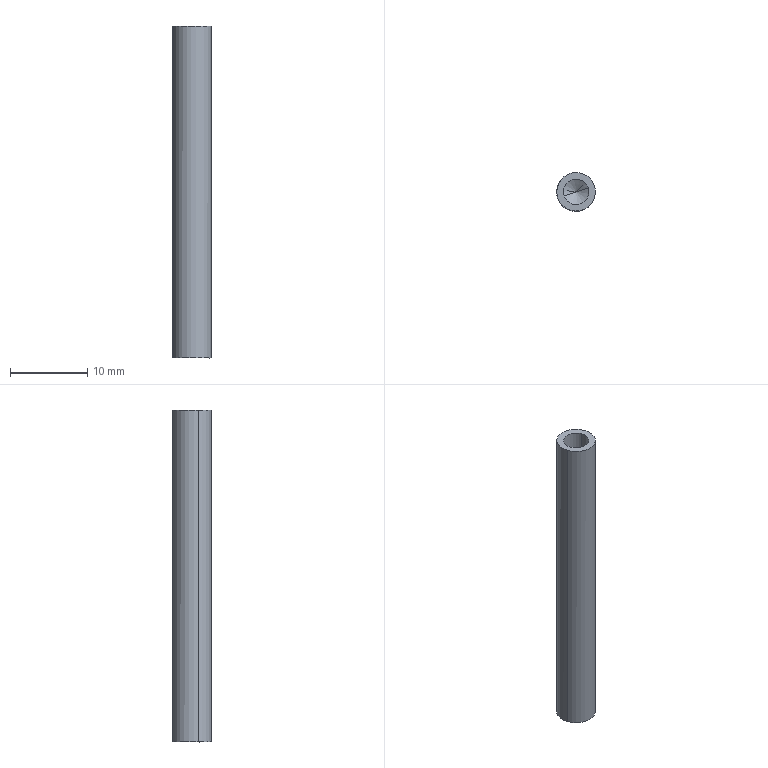Part | SolidWorks | features BaseBody 1 | 1 solid | 12 faces | box 5.036 x 5.019 x 43.005 mm | volume 701.802 mm3 | cylinder 6 | cone 4 | plane 2 | commonest cylinder face diameters 3.3 x4 5 x2
STEP:
#1=CARTESIAN_POINT('',(-258.909,167.447,-138.014));
#2=VERTEX_POINT('',#1);
#3=CARTESIAN_POINT('',(-260.471,166.914,-139.005));
#4=VERTEX_POINT('',#3);
#5=CARTESIAN_POINT('',(-258.909,167.447,-138.014));
#6=DIRECTION('',(-0.8116,-0.2768,-0.5145));
#7=VECTOR('',#6,1000.);
#8=LINE('',#5,#7);
#9=EDGE_CURVE('',#2,#4,#8,.T.);
#10=ORIENTED_EDGE('',*,*,#9,.F.);
#11=CARTESIAN_POINT('',(-262.031,166.381,-138.012));
#12=VERTEX_POINT('',#11);
#13=CARTESIAN_POINT('',(-260.47,166.914,-138.013));
#14=DIRECTION('',(-0.0008339,0.0004454,-1.));
#15=DIRECTION('',(-0.9463,-0.3232,0.0006452));
#16=AXIS2_PLACEMENT_3D('',#13,#14,#15);
#17=CIRCLE('',#16,1.65);
#18=EDGE_CURVE('',#12,#2,#17,.T.);
#19=ORIENTED_EDGE('',*,*,#18,.F.);
#20=CARTESIAN_POINT('',(-262.031,166.381,-138.012));
#21=DIRECTION('',(0.8107,0.2773,-0.5156));
#22=VECTOR('',#21,1000.);
#23=LINE('',#20,#22);
#24=EDGE_CURVE('',#12,#4,#23,.T.);
#25=ORIENTED_EDGE('',*,*,#24,.T.);
#26=EDGE_LOOP('',(#10,#19,#25));
#27=FACE_OUTER_BOUND('',#26,.T.);
#28=CARTESIAN_POINT('',(-260.47,166.914,-138.478));
#29=DIRECTION('',(0.0008339,-0.0004454,1.));
#30=DIRECTION('',(0.9463,0.3232,-0.0006452));
#31=AXIS2_PLACEMENT_3D('',#28,#29,#30);
#32=CONICAL_SURFACE('',#31,0.8764,1.03);
#33=ADVANCED_FACE('',(#27),#32,.F.);
#34=ORIENTED_EDGE('',*,*,#24,.F.);
#35=CARTESIAN_POINT('',(-260.47,166.914,-138.013));
#36=DIRECTION('',(-0.0008339,0.0004454,-1.));
#37=DIRECTION('',(0.9463,0.3232,-0.0006452));
#38=AXIS2_PLACEMENT_3D('',#35,#36,#37);
#39=CIRCLE('',#38,1.65);
#40=EDGE_CURVE('',#2,#12,#39,.T.);
#41=ORIENTED_EDGE('',*,*,#40,.F.);
#42=ORIENTED_EDGE('',*,*,#9,.T.);
#43=EDGE_LOOP('',(#34,#41,#42));
#44=FACE_OUTER_BOUND('',#43,.T.);
#45=CARTESIAN_POINT('',(-260.47,166.914,-138.478));
#46=DIRECTION('',(0.0008339,-0.0004454,1.));
#47=DIRECTION('',(0.9463,0.3232,-0.0006452));
#48=AXIS2_PLACEMENT_3D('',#45,#46,#47);
#49=CONICAL_SURFACE('',#48,0.8764,1.03);
#50=ADVANCED_FACE('',(#44),#49,.F.);
#51=CARTESIAN_POINT('',(-262.025,166.377,-130.012));
#52=VERTEX_POINT('',#51);
#53=CARTESIAN_POINT('',(-262.025,166.377,-130.012));
#54=DIRECTION('',(-0.0008339,0.0004454,-1.));
#55=VECTOR('',#54,1000.);
#56=LINE('',#53,#55);
#57=EDGE_CURVE('',#52,#12,#56,.T.);
#58=ORIENTED_EDGE('',*,*,#57,.F.);
#59=CARTESIAN_POINT('',(-258.902,167.444,-130.014));
#60=VERTEX_POINT('',#59);
#61=CARTESIAN_POINT('',(-260.463,166.91,-130.013));
#62=DIRECTION('',(0.0008339,-0.0004454,1.));
#63=DIRECTION('',(-0.9463,-0.3232,0.0006452));
#64=AXIS2_PLACEMENT_3D('',#61,#62,#63);
#65=CIRCLE('',#64,1.65);
#66=EDGE_CURVE('',#52,#60,#65,.T.);
#67=ORIENTED_EDGE('',*,*,#66,.T.);
#68=CARTESIAN_POINT('',(-258.902,167.444,-130.014));
#69=DIRECTION('',(-0.0008339,0.0004454,-1.));
#70=VECTOR('',#69,1000.);
#71=LINE('',#68,#70);
#72=EDGE_CURVE('',#60,#2,#71,.T.);
#73=ORIENTED_EDGE('',*,*,#72,.T.);
#74=ORIENTED_EDGE('',*,*,#40,.T.);
#75=EDGE_LOOP('',(#58,#67,#73,#74));
#76=FACE_OUTER_BOUND('',#75,.T.);
#77=CARTESIAN_POINT('',(-260.463,166.91,-130.013));
#78=DIRECTION('',(0.0008339,-0.0004454,1.));
#79=DIRECTION('',(0.9463,0.3232,-0.0006452));
#80=AXIS2_PLACEMENT_3D('',#77,#78,#79);
#81=CYLINDRICAL_SURFACE('',#80,1.65);
#82=ADVANCED_FACE('',(#76),#81,.F.);
#83=ORIENTED_EDGE('',*,*,#18,.T.);
#84=ORIENTED_EDGE('',*,*,#72,.F.);
#85=CARTESIAN_POINT('',(-260.463,166.91,-130.013));
#86=DIRECTION('',(0.0008339,-0.0004454,1.));
#87=DIRECTION('',(0.9463,0.3232,-0.0006452));
#88=AXIS2_PLACEMENT_3D('',#85,#86,#87);
#89=CIRCLE('',#88,1.65);
#90=EDGE_CURVE('',#60,#52,#89,.T.);
#91=ORIENTED_EDGE('',*,*,#90,.T.);
#92=ORIENTED_EDGE('',*,*,#57,.T.);
#93=EDGE_LOOP('',(#83,#84,#91,#92));
#94=FACE_OUTER_BOUND('',#93,.T.);
#95=CARTESIAN_POINT('',(-260.463,166.91,-130.013));
#96=DIRECTION('',(0.0008339,-0.0004454,1.));
#97=DIRECTION('',(0.9463,0.3232,-0.0006452));
#98=AXIS2_PLACEMENT_3D('',#95,#96,#97);
#99=CYLINDRICAL_SURFACE('',#98,1.65);
#100=ADVANCED_FACE('',(#94),#99,.F.);
#101=ORIENTED_EDGE('',*,*,#66,.F.);
#102=ORIENTED_EDGE('',*,*,#90,.F.);
#103=EDGE_LOOP('',(#101,#102));
#104=FACE_BOUND('',#103,.T.);
#105=CARTESIAN_POINT('',(-262.829,166.102,-130.011));
#106=VERTEX_POINT('',#105);
#107=CARTESIAN_POINT('',(-258.098,167.718,-130.015));
#108=VERTEX_POINT('',#107);
#109=CARTESIAN_POINT('',(-260.463,166.91,-130.013));
#110=DIRECTION('',(-0.0008339,0.0004454,-1.));
#111=DIRECTION('',(-0.9463,-0.3232,0.0006452));
#112=AXIS2_PLACEMENT_3D('',#109,#110,#111);
#113=CIRCLE('',#112,2.5);
#114=EDGE_CURVE('',#106,#108,#113,.T.);
#115=ORIENTED_EDGE('',*,*,#114,.F.);
#116=CARTESIAN_POINT('',(-260.463,166.91,-130.013));
#117=DIRECTION('',(-0.0008339,0.0004454,-1.));
#118=DIRECTION('',(0.9463,0.3232,-0.0006452));
#119=AXIS2_PLACEMENT_3D('',#116,#117,#118);
#120=CIRCLE('',#119,2.5);
#121=EDGE_CURVE('',#108,#106,#120,.T.);
#122=ORIENTED_EDGE('',*,*,#121,.F.);
#123=EDGE_LOOP('',(#115,#122));
#124=FACE_OUTER_BOUND('',#123,.T.);
#125=CARTESIAN_POINT('',(-260.463,166.91,-130.013));
#126=DIRECTION('',(0.0008339,-0.0004454,1.));
#127=DIRECTION('',(-0.4711,-0.8821,0.));
#128=AXIS2_PLACEMENT_3D('',#125,#126,#127);
#129=PLANE('',#128);
#130=ADVANCED_FACE('',(#104,#124),#129,.T.);
#131=ORIENTED_EDGE('',*,*,#121,.T.);
#132=CARTESIAN_POINT('',(-262.865,166.121,-173.011));
#133=VERTEX_POINT('',#132);
#134=CARTESIAN_POINT('',(-262.865,166.121,-173.011));
#135=DIRECTION('',(0.0008339,-0.0004454,1.));
#136=VECTOR('',#135,1000.);
#137=LINE('',#134,#136);
#138=EDGE_CURVE('',#133,#106,#137,.T.);
#139=ORIENTED_EDGE('',*,*,#138,.F.);
#140=CARTESIAN_POINT('',(-258.133,167.737,-173.015));
#141=VERTEX_POINT('',#140);
#142=CARTESIAN_POINT('',(-260.499,166.929,-173.013));
#143=DIRECTION('',(0.0008339,-0.0004454,1.));
#144=DIRECTION('',(-0.9463,-0.3232,0.0006452));
#145=AXIS2_PLACEMENT_3D('',#142,#143,#144);
#146=CIRCLE('',#145,2.5);
#147=EDGE_CURVE('',#133,#141,#146,.T.);
#148=ORIENTED_EDGE('',*,*,#147,.T.);
#149=CARTESIAN_POINT('',(-258.133,167.737,-173.015));
#150=DIRECTION('',(0.0008339,-0.0004454,1.));
#151=VECTOR('',#150,1000.);
#152=LINE('',#149,#151);
#153=EDGE_CURVE('',#141,#108,#152,.T.);
#154=ORIENTED_EDGE('',*,*,#153,.T.);
#155=EDGE_LOOP('',(#131,#139,#148,#154));
#156=FACE_OUTER_BOUND('',#155,.T.);
#157=CARTESIAN_POINT('',(-260.463,166.91,-130.013));
#158=DIRECTION('',(-0.0008339,0.0004454,-1.));
#159=DIRECTION('',(-0.9463,-0.3232,0.0006452));
#160=AXIS2_PLACEMENT_3D('',#157,#158,#159);
#161=CYLINDRICAL_SURFACE('',#160,2.5);
#162=ADVANCED_FACE('',(#156),#161,.T.);
#163=ORIENTED_EDGE('',*,*,#153,.F.);
#164=CARTESIAN_POINT('',(-260.499,166.929,-173.013));
#165=DIRECTION('',(0.0008339,-0.0004454,1.));
#166=DIRECTION('',(0.9463,0.3232,-0.0006452));
#167=AXIS2_PLACEMENT_3D('',#164,#165,#166);
#168=CIRCLE('',#167,2.5);
#169=EDGE_CURVE('',#141,#133,#168,.T.);
#170=ORIENTED_EDGE('',*,*,#169,.T.);
#171=ORIENTED_EDGE('',*,*,#138,.T.);
#172=ORIENTED_EDGE('',*,*,#114,.T.);
#173=EDGE_LOOP('',(#163,#170,#171,#172));
#174=FACE_OUTER_BOUND('',#173,.T.);
#175=CARTESIAN_POINT('',(-260.463,166.91,-130.013));
#176=DIRECTION('',(-0.0008339,0.0004454,-1.));
#177=DIRECTION('',(-0.9463,-0.3232,0.0006452));
#178=AXIS2_PLACEMENT_3D('',#175,#176,#177);
#179=CYLINDRICAL_SURFACE('',#178,2.5);
#180=ADVANCED_FACE('',(#174),#179,.T.);
#181=CARTESIAN_POINT('',(-258.938,167.463,-173.014));
#182=VERTEX_POINT('',#181);
#183=CARTESIAN_POINT('',(-262.061,166.396,-173.012));
#184=VERTEX_POINT('',#183);
#185=CARTESIAN_POINT('',(-260.499,166.929,-173.013));
#186=DIRECTION('',(-0.0008339,0.0004454,-1.));
#187=DIRECTION('',(0.9463,0.3232,-0.0006452));
#188=AXIS2_PLACEMENT_3D('',#185,#186,#187);
#189=CIRCLE('',#188,1.65);
#190=EDGE_CURVE('',#182,#184,#189,.T.);
#191=ORIENTED_EDGE('',*,*,#190,.F.);
#192=CARTESIAN_POINT('',(-260.499,166.929,-173.013));
#193=DIRECTION('',(-0.0008339,0.0004454,-1.));
#194=DIRECTION('',(-0.9463,-0.3232,0.0006452));
#195=AXIS2_PLACEMENT_3D('',#192,#193,#194);
#196=CIRCLE('',#195,1.65);
#197=EDGE_CURVE('',#184,#182,#196,.T.);
#198=ORIENTED_EDGE('',*,*,#197,.F.);
#199=EDGE_LOOP('',(#191,#198));
#200=FACE_BOUND('',#199,.T.);
#201=ORIENTED_EDGE('',*,*,#169,.F.);
#202=ORIENTED_EDGE('',*,*,#147,.F.);
#203=EDGE_LOOP('',(#201,#202));
#204=FACE_OUTER_BOUND('',#203,.T.);
#205=CARTESIAN_POINT('',(-260.499,166.929,-173.013));
#206=DIRECTION('',(0.0008339,-0.0004454,1.));
#207=DIRECTION('',(-0.4711,-0.8821,0.));
#208=AXIS2_PLACEMENT_3D('',#205,#206,#207);
#209=PLANE('',#208);
#210=ADVANCED_FACE('',(#200,#204),#209,.F.);
#211=CARTESIAN_POINT('',(-258.931,167.459,-165.014));
#212=VERTEX_POINT('',#211);
#213=CARTESIAN_POINT('',(-262.054,166.393,-165.012));
#214=VERTEX_POINT('',#213);
#215=CARTESIAN_POINT('',(-260.493,166.926,-165.013));
#216=DIRECTION('',(0.0008339,-0.0004454,1.));
#217=DIRECTION('',(0.9463,0.3232,-0.0006452));
#218=AXIS2_PLACEMENT_3D('',#215,#216,#217);
#219=CIRCLE('',#218,1.65);
#220=EDGE_CURVE('',#212,#214,#219,.T.);
#221=ORIENTED_EDGE('',*,*,#220,.T.);
#222=CARTESIAN_POINT('',(-262.061,166.396,-173.012));
#223=DIRECTION('',(0.0008339,-0.0004454,1.));
#224=VECTOR('',#223,1000.);
#225=LINE('',#222,#224);
#226=EDGE_CURVE('',#184,#214,#225,.T.);
#227=ORIENTED_EDGE('',*,*,#226,.F.);
#228=ORIENTED_EDGE('',*,*,#197,.T.);
#229=CARTESIAN_POINT('',(-258.938,167.463,-173.014));
#230=DIRECTION('',(0.0008339,-0.0004454,1.));
#231=VECTOR('',#230,1000.);
#232=LINE('',#229,#231);
#233=EDGE_CURVE('',#182,#212,#232,.T.);
#234=ORIENTED_EDGE('',*,*,#233,.T.);
#235=EDGE_LOOP('',(#221,#227,#228,#234));
#236=FACE_OUTER_BOUND('',#235,.T.);
#237=CARTESIAN_POINT('',(-260.499,166.929,-173.013));
#238=DIRECTION('',(-0.0008339,0.0004454,-1.));
#239=DIRECTION('',(-0.9463,-0.3232,0.0006452));
#240=AXIS2_PLACEMENT_3D('',#237,#238,#239);
#241=CYLINDRICAL_SURFACE('',#240,1.65);
#242=ADVANCED_FACE('',(#236),#241,.F.);
#243=ORIENTED_EDGE('',*,*,#233,.F.);
#244=ORIENTED_EDGE('',*,*,#190,.T.);
#245=ORIENTED_EDGE('',*,*,#226,.T.);
#246=CARTESIAN_POINT('',(-260.493,166.926,-165.013));
#247=DIRECTION('',(0.0008339,-0.0004454,1.));
#248=DIRECTION('',(-0.9463,-0.3232,0.0006452));
#249=AXIS2_PLACEMENT_3D('',#246,#247,#248);
#250=CIRCLE('',#249,1.65);
#251=EDGE_CURVE('',#214,#212,#250,.T.);
#252=ORIENTED_EDGE('',*,*,#251,.T.);
#253=EDGE_LOOP('',(#243,#244,#245,#252));
#254=FACE_OUTER_BOUND('',#253,.T.);
#255=CARTESIAN_POINT('',(-260.499,166.929,-173.013));
#256=DIRECTION('',(-0.0008339,0.0004454,-1.));
#257=DIRECTION('',(-0.9463,-0.3232,0.0006452));
#258=AXIS2_PLACEMENT_3D('',#255,#256,#257);
#259=CYLINDRICAL_SURFACE('',#258,1.65);
#260=ADVANCED_FACE('',(#254),#259,.F.);
#261=CARTESIAN_POINT('',(-260.492,166.925,-164.022));
#262=VERTEX_POINT('',#261);
#263=CARTESIAN_POINT('',(-258.931,167.459,-165.014));
#264=DIRECTION('',(-0.8107,-0.2773,0.5156));
#265=VECTOR('',#264,1000.);
#266=LINE('',#263,#265);
#267=EDGE_CURVE('',#212,#262,#266,.T.);
#268=ORIENTED_EDGE('',*,*,#267,.F.);
#269=ORIENTED_EDGE('',*,*,#251,.F.);
#270=CARTESIAN_POINT('',(-262.054,166.393,-165.012));
#271=DIRECTION('',(0.8116,0.2768,0.5145));
#272=VECTOR('',#271,1000.);
#273=LINE('',#270,#272);
#274=EDGE_CURVE('',#214,#262,#273,.T.);
#275=ORIENTED_EDGE('',*,*,#274,.T.);
#276=EDGE_LOOP('',(#268,#269,#275));
#277=FACE_OUTER_BOUND('',#276,.T.);
#278=CARTESIAN_POINT('',(-260.492,166.926,-164.548));
#279=DIRECTION('',(-0.0008339,0.0004454,-1.));
#280=DIRECTION('',(-0.9463,-0.3232,0.0006452));
#281=AXIS2_PLACEMENT_3D('',#278,#279,#280);
#282=CONICAL_SURFACE('',#281,0.8764,1.03);
#283=ADVANCED_FACE('',(#277),#282,.F.);
#284=ORIENTED_EDGE('',*,*,#274,.F.);
#285=ORIENTED_EDGE('',*,*,#220,.F.);
#286=ORIENTED_EDGE('',*,*,#267,.T.);
#287=EDGE_LOOP('',(#284,#285,#286));
#288=FACE_OUTER_BOUND('',#287,.T.);
#289=CARTESIAN_POINT('',(-260.492,166.926,-164.548));
#290=DIRECTION('',(-0.0008339,0.0004454,-1.));
#291=DIRECTION('',(-0.9463,-0.3232,0.0006452));
#292=AXIS2_PLACEMENT_3D('',#289,#290,#291);
#293=CONICAL_SURFACE('',#292,0.8764,1.03);
#294=ADVANCED_FACE('',(#288),#293,.F.);
#295=CLOSED_SHELL('',(#33,#50,#82,#100,#130,#162,#180,#210,#242,#260,#283,#294));
#296=MANIFOLD_SOLID_BREP('',#295);
#297=CARTESIAN_POINT('',(0.,0.,0.));
#298=DIRECTION('',(0.,0.,1.));
#299=DIRECTION('',(1.,0.,0.));
#300=AXIS2_PLACEMENT_3D('',#297,#298,#299);
#301=(LENGTH_UNIT()NAMED_UNIT(*)SI_UNIT(.MILLI.,.METRE.));
#302=UNCERTAINTY_MEASURE_WITH_UNIT(LENGTH_MEASURE(0.00001),#301,'','');
#303=(NAMED_UNIT(*)PLANE_ANGLE_UNIT()SI_UNIT($,.RADIAN.));
#304=(NAMED_UNIT(*)SI_UNIT($,.STERADIAN.)SOLID_ANGLE_UNIT());
#305=(GEOMETRIC_REPRESENTATION_CONTEXT(3)GLOBAL_UNCERTAINTY_ASSIGNED_CONTEXT((#302))GLOBAL_UNIT_ASSIGNED_CONTEXT((#301,#303,#304))REPRESENTATION_CONTEXT('',''));
#306=ADVANCED_BREP_SHAPE_REPRESENTATION('',(#296,#300),#305);